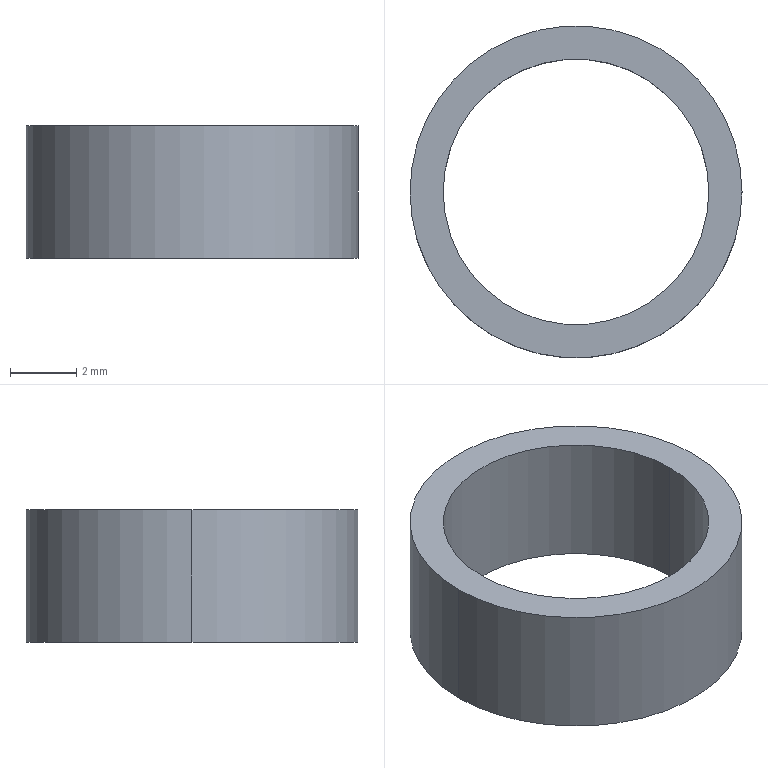Part | NX | features BREP 1 | 1 solid | 6 faces | box 10 x 10 x 4 mm | volume 113.097 mm3 | cylinder 4 | plane 2 | commonest cylinder face diameters 8 x2 10 x2
STEP:
#1=CARTESIAN_POINT('',(-4.,0.,4.));
#2=VERTEX_POINT('',#1);
#3=CARTESIAN_POINT('',(4.,0.,4.));
#4=VERTEX_POINT('',#3);
#5=CARTESIAN_POINT('',(0.,0.,4.));
#6=DIRECTION('',(0.,0.,1.));
#7=DIRECTION('',(1.,0.,0.));
#8=AXIS2_PLACEMENT_3D('',#5,#6,#7);
#9=CIRCLE('',#8,4.);
#10=EDGE_CURVE('',#2,#4,#9,.T.);
#11=ORIENTED_EDGE('',*,*,#10,.T.);
#12=CARTESIAN_POINT('',(4.,0.,0.));
#13=VERTEX_POINT('',#12);
#14=CARTESIAN_POINT('',(4.,0.,4.));
#15=DIRECTION('',(0.,0.,-1.));
#16=VECTOR('',#15,1000.);
#17=LINE('',#14,#16);
#18=EDGE_CURVE('',#4,#13,#17,.T.);
#19=ORIENTED_EDGE('',*,*,#18,.T.);
#20=CARTESIAN_POINT('',(-4.,0.,0.));
#21=VERTEX_POINT('',#20);
#22=CARTESIAN_POINT('',(0.,0.,0.));
#23=DIRECTION('',(0.,0.,1.));
#24=DIRECTION('',(1.,0.,0.));
#25=AXIS2_PLACEMENT_3D('',#22,#23,#24);
#26=CIRCLE('',#25,4.);
#27=EDGE_CURVE('',#21,#13,#26,.T.);
#28=ORIENTED_EDGE('',*,*,#27,.F.);
#29=CARTESIAN_POINT('',(-4.,0.,4.));
#30=DIRECTION('',(0.,0.,-1.));
#31=VECTOR('',#30,1000.);
#32=LINE('',#29,#31);
#33=EDGE_CURVE('',#2,#21,#32,.T.);
#34=ORIENTED_EDGE('',*,*,#33,.F.);
#35=EDGE_LOOP('',(#11,#19,#28,#34));
#36=FACE_BOUND('',#35,.T.);
#37=CARTESIAN_POINT('',(0.,0.,4.));
#38=DIRECTION('',(0.,0.,-1.));
#39=DIRECTION('',(-1.,0.,0.));
#40=AXIS2_PLACEMENT_3D('',#37,#38,#39);
#41=CYLINDRICAL_SURFACE('',#40,4.);
#42=ADVANCED_FACE('',(#36),#41,.F.);
#43=CARTESIAN_POINT('',(5.,0.,4.));
#44=VERTEX_POINT('',#43);
#45=CARTESIAN_POINT('',(-5.,0.,4.));
#46=VERTEX_POINT('',#45);
#47=CARTESIAN_POINT('',(0.,0.,4.));
#48=DIRECTION('',(0.,0.,1.));
#49=DIRECTION('',(1.,0.,0.));
#50=AXIS2_PLACEMENT_3D('',#47,#48,#49);
#51=CIRCLE('',#50,5.);
#52=EDGE_CURVE('',#44,#46,#51,.T.);
#53=ORIENTED_EDGE('',*,*,#52,.F.);
#54=CARTESIAN_POINT('',(5.,0.,0.));
#55=VERTEX_POINT('',#54);
#56=CARTESIAN_POINT('',(5.,0.,4.));
#57=DIRECTION('',(0.,0.,-1.));
#58=VECTOR('',#57,1000.);
#59=LINE('',#56,#58);
#60=EDGE_CURVE('',#44,#55,#59,.T.);
#61=ORIENTED_EDGE('',*,*,#60,.T.);
#62=CARTESIAN_POINT('',(-5.,0.,0.));
#63=VERTEX_POINT('',#62);
#64=CARTESIAN_POINT('',(0.,0.,0.));
#65=DIRECTION('',(0.,0.,1.));
#66=DIRECTION('',(1.,0.,0.));
#67=AXIS2_PLACEMENT_3D('',#64,#65,#66);
#68=CIRCLE('',#67,5.);
#69=EDGE_CURVE('',#55,#63,#68,.T.);
#70=ORIENTED_EDGE('',*,*,#69,.T.);
#71=CARTESIAN_POINT('',(-5.,0.,4.));
#72=DIRECTION('',(0.,0.,-1.));
#73=VECTOR('',#72,1000.);
#74=LINE('',#71,#73);
#75=EDGE_CURVE('',#46,#63,#74,.T.);
#76=ORIENTED_EDGE('',*,*,#75,.F.);
#77=EDGE_LOOP('',(#53,#61,#70,#76));
#78=FACE_BOUND('',#77,.T.);
#79=CARTESIAN_POINT('',(0.,0.,4.));
#80=DIRECTION('',(0.,0.,-1.));
#81=DIRECTION('',(-1.,0.,0.));
#82=AXIS2_PLACEMENT_3D('',#79,#80,#81);
#83=CYLINDRICAL_SURFACE('',#82,5.);
#84=ADVANCED_FACE('',(#78),#83,.T.);
#85=CARTESIAN_POINT('',(0.,0.,4.));
#86=DIRECTION('',(0.,0.,1.));
#87=DIRECTION('',(1.,0.,0.));
#88=AXIS2_PLACEMENT_3D('',#85,#86,#87);
#89=CIRCLE('',#88,5.);
#90=EDGE_CURVE('',#46,#44,#89,.T.);
#91=ORIENTED_EDGE('',*,*,#90,.T.);
#92=ORIENTED_EDGE('',*,*,#52,.T.);
#93=EDGE_LOOP('',(#91,#92));
#94=FACE_BOUND('',#93,.T.);
#95=ORIENTED_EDGE('',*,*,#10,.F.);
#96=CARTESIAN_POINT('',(0.,0.,4.));
#97=DIRECTION('',(0.,0.,1.));
#98=DIRECTION('',(1.,0.,0.));
#99=AXIS2_PLACEMENT_3D('',#96,#97,#98);
#100=CIRCLE('',#99,4.);
#101=EDGE_CURVE('',#4,#2,#100,.T.);
#102=ORIENTED_EDGE('',*,*,#101,.F.);
#103=EDGE_LOOP('',(#95,#102));
#104=FACE_BOUND('',#103,.T.);
#105=CARTESIAN_POINT('',(0.,0.,4.));
#106=DIRECTION('',(0.,0.,1.));
#107=DIRECTION('',(1.,0.,0.));
#108=AXIS2_PLACEMENT_3D('',#105,#106,#107);
#109=PLANE('',#108);
#110=ADVANCED_FACE('',(#94,#104),#109,.T.);
#111=CARTESIAN_POINT('',(0.,0.,0.));
#112=DIRECTION('',(0.,0.,1.));
#113=DIRECTION('',(1.,0.,0.));
#114=AXIS2_PLACEMENT_3D('',#111,#112,#113);
#115=CIRCLE('',#114,5.);
#116=EDGE_CURVE('',#63,#55,#115,.T.);
#117=ORIENTED_EDGE('',*,*,#116,.F.);
#118=ORIENTED_EDGE('',*,*,#69,.F.);
#119=EDGE_LOOP('',(#117,#118));
#120=FACE_BOUND('',#119,.T.);
#121=ORIENTED_EDGE('',*,*,#27,.T.);
#122=CARTESIAN_POINT('',(0.,0.,0.));
#123=DIRECTION('',(0.,0.,1.));
#124=DIRECTION('',(1.,0.,0.));
#125=AXIS2_PLACEMENT_3D('',#122,#123,#124);
#126=CIRCLE('',#125,4.);
#127=EDGE_CURVE('',#13,#21,#126,.T.);
#128=ORIENTED_EDGE('',*,*,#127,.T.);
#129=EDGE_LOOP('',(#121,#128));
#130=FACE_BOUND('',#129,.T.);
#131=CARTESIAN_POINT('',(0.,0.,0.));
#132=DIRECTION('',(0.,0.,1.));
#133=DIRECTION('',(1.,0.,0.));
#134=AXIS2_PLACEMENT_3D('',#131,#132,#133);
#135=PLANE('',#134);
#136=ADVANCED_FACE('',(#120,#130),#135,.F.);
#137=ORIENTED_EDGE('',*,*,#60,.F.);
#138=ORIENTED_EDGE('',*,*,#90,.F.);
#139=ORIENTED_EDGE('',*,*,#75,.T.);
#140=ORIENTED_EDGE('',*,*,#116,.T.);
#141=EDGE_LOOP('',(#137,#138,#139,#140));
#142=FACE_BOUND('',#141,.T.);
#143=CARTESIAN_POINT('',(0.,0.,4.));
#144=DIRECTION('',(0.,0.,-1.));
#145=DIRECTION('',(-1.,0.,0.));
#146=AXIS2_PLACEMENT_3D('',#143,#144,#145);
#147=CYLINDRICAL_SURFACE('',#146,5.);
#148=ADVANCED_FACE('',(#142),#147,.T.);
#149=ORIENTED_EDGE('',*,*,#18,.F.);
#150=ORIENTED_EDGE('',*,*,#101,.T.);
#151=ORIENTED_EDGE('',*,*,#33,.T.);
#152=ORIENTED_EDGE('',*,*,#127,.F.);
#153=EDGE_LOOP('',(#149,#150,#151,#152));
#154=FACE_BOUND('',#153,.T.);
#155=CARTESIAN_POINT('',(0.,0.,4.));
#156=DIRECTION('',(0.,0.,-1.));
#157=DIRECTION('',(-1.,0.,0.));
#158=AXIS2_PLACEMENT_3D('',#155,#156,#157);
#159=CYLINDRICAL_SURFACE('',#158,4.);
#160=ADVANCED_FACE('',(#154),#159,.F.);
#161=CLOSED_SHELL('',(#42,#84,#110,#136,#148,#160));
#162=MANIFOLD_SOLID_BREP('',#161);
#163=(LENGTH_UNIT()NAMED_UNIT(*)SI_UNIT(.MILLI.,.METRE.));
#164=UNCERTAINTY_MEASURE_WITH_UNIT(LENGTH_MEASURE(0.00001),#163,'','');
#165=(NAMED_UNIT(*)PLANE_ANGLE_UNIT()SI_UNIT($,.RADIAN.));
#166=(NAMED_UNIT(*)SI_UNIT($,.STERADIAN.)SOLID_ANGLE_UNIT());
#167=(GEOMETRIC_REPRESENTATION_CONTEXT(3)GLOBAL_UNCERTAINTY_ASSIGNED_CONTEXT((#164))GLOBAL_UNIT_ASSIGNED_CONTEXT((#163,#165,#166))REPRESENTATION_CONTEXT('',''));
#168=ADVANCED_BREP_SHAPE_REPRESENTATION('',(#162),#167);